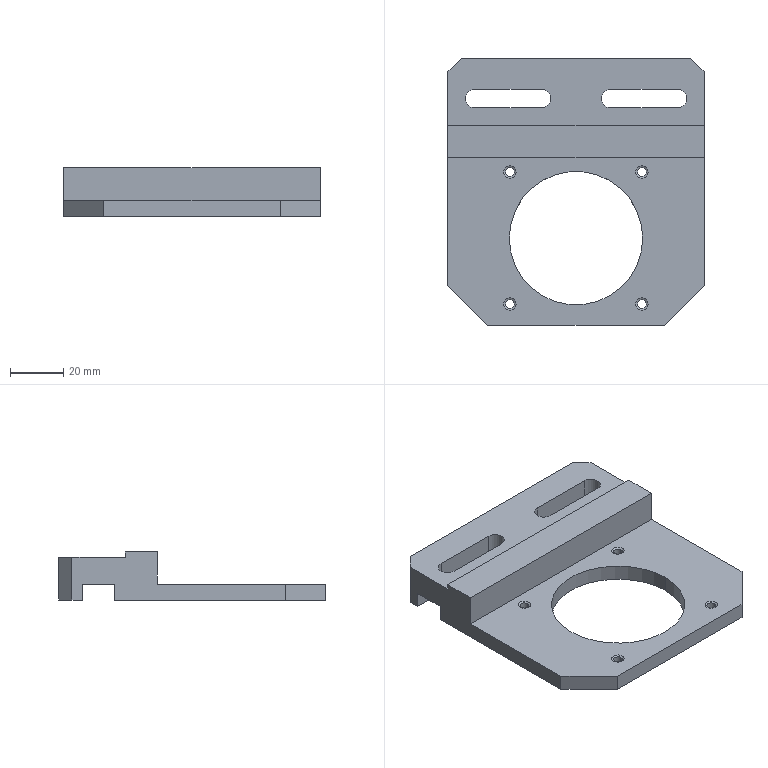Part | NX | 1 solid | 46 faces | box 96 x 100 x 18 mm | volume 70500 mm3 | plane 22 | cylinder 16 | cone 8 | commonest cylinder face diameters 3.3 x8 7 x6 50 x2
STEP:
#1=CARTESIAN_POINT('',(48.,41.,-8.));
#2=VERTEX_POINT('',#1);
#3=CARTESIAN_POINT('',(48.,45.,-8.));
#4=VERTEX_POINT('',#3);
#5=CARTESIAN_POINT('',(48.,0.,-8.));
#6=DIRECTION('',(0.,1.,0.));
#7=VECTOR('',#6,1000.);
#8=LINE('',#5,#7);
#9=EDGE_CURVE('',#2,#4,#8,.T.);
#10=ORIENTED_EDGE('',*,*,#9,.F.);
#11=CARTESIAN_POINT('',(-48.,41.,-8.));
#12=VERTEX_POINT('',#11);
#13=CARTESIAN_POINT('',(0.,41.,-8.));
#14=DIRECTION('',(-1.,0.,0.));
#15=VECTOR('',#14,1000.);
#16=LINE('',#13,#15);
#17=EDGE_CURVE('',#2,#12,#16,.T.);
#18=ORIENTED_EDGE('',*,*,#17,.T.);
#19=CARTESIAN_POINT('',(-48.,45.,-8.));
#20=VERTEX_POINT('',#19);
#21=CARTESIAN_POINT('',(-48.,0.,-8.));
#22=DIRECTION('',(0.,1.,0.));
#23=VECTOR('',#22,1000.);
#24=LINE('',#21,#23);
#25=EDGE_CURVE('',#12,#20,#24,.T.);
#26=ORIENTED_EDGE('',*,*,#25,.T.);
#27=CARTESIAN_POINT('',(-43.,50.,-8.));
#28=VERTEX_POINT('',#27);
#29=CARTESIAN_POINT('',(-93.,0.,-8.));
#30=DIRECTION('',(0.7071,0.7071,0.));
#31=VECTOR('',#30,1000.);
#32=LINE('',#29,#31);
#33=EDGE_CURVE('',#20,#28,#32,.T.);
#34=ORIENTED_EDGE('',*,*,#33,.T.);
#35=CARTESIAN_POINT('',(43.,50.,-8.));
#36=VERTEX_POINT('',#35);
#37=CARTESIAN_POINT('',(0.,50.,-8.));
#38=DIRECTION('',(-1.,0.,0.));
#39=VECTOR('',#38,1000.);
#40=LINE('',#37,#39);
#41=EDGE_CURVE('',#36,#28,#40,.T.);
#42=ORIENTED_EDGE('',*,*,#41,.F.);
#43=CARTESIAN_POINT('',(93.,0.,-8.));
#44=DIRECTION('',(0.7071,-0.7071,0.));
#45=VECTOR('',#44,1000.);
#46=LINE('',#43,#45);
#47=EDGE_CURVE('',#36,#4,#46,.T.);
#48=ORIENTED_EDGE('',*,*,#47,.T.);
#49=EDGE_LOOP('',(#10,#18,#26,#34,#42,#48));
#50=FACE_BOUND('',#49,.T.);
#51=CARTESIAN_POINT('',(0.,0.,-8.));
#52=DIRECTION('',(0.,0.,1.));
#53=DIRECTION('',(1.,0.,0.));
#54=AXIS2_PLACEMENT_3D('',#51,#52,#53);
#55=PLANE('',#54);
#56=ADVANCED_FACE('',(#50),#55,.F.);
#57=CARTESIAN_POINT('',(-48.,45.,8.));
#58=VERTEX_POINT('',#57);
#59=CARTESIAN_POINT('',(-48.,45.,0.));
#60=DIRECTION('',(0.,0.,1.));
#61=VECTOR('',#60,1000.);
#62=LINE('',#59,#61);
#63=EDGE_CURVE('',#20,#58,#62,.T.);
#64=ORIENTED_EDGE('',*,*,#63,.F.);
#65=ORIENTED_EDGE('',*,*,#25,.F.);
#66=CARTESIAN_POINT('',(-48.,41.,-2.));
#67=VERTEX_POINT('',#66);
#68=CARTESIAN_POINT('',(-48.,41.,0.));
#69=DIRECTION('',(0.,0.,-1.));
#70=VECTOR('',#69,1000.);
#71=LINE('',#68,#70);
#72=EDGE_CURVE('',#67,#12,#71,.T.);
#73=ORIENTED_EDGE('',*,*,#72,.F.);
#74=CARTESIAN_POINT('',(-48.,29.,-2.));
#75=VERTEX_POINT('',#74);
#76=CARTESIAN_POINT('',(-48.,0.,-2.));
#77=DIRECTION('',(0.,-1.,0.));
#78=VECTOR('',#77,1000.);
#79=LINE('',#76,#78);
#80=EDGE_CURVE('',#67,#75,#79,.T.);
#81=ORIENTED_EDGE('',*,*,#80,.T.);
#82=CARTESIAN_POINT('',(-48.,29.,-8.));
#83=VERTEX_POINT('',#82);
#84=CARTESIAN_POINT('',(-48.,29.,0.));
#85=DIRECTION('',(0.,0.,1.));
#86=VECTOR('',#85,1000.);
#87=LINE('',#84,#86);
#88=EDGE_CURVE('',#83,#75,#87,.T.);
#89=ORIENTED_EDGE('',*,*,#88,.F.);
#90=CARTESIAN_POINT('',(-48.,-35.,-8.));
#91=VERTEX_POINT('',#90);
#92=CARTESIAN_POINT('',(-48.,0.,-8.));
#93=DIRECTION('',(0.,1.,0.));
#94=VECTOR('',#93,1000.);
#95=LINE('',#92,#94);
#96=EDGE_CURVE('',#91,#83,#95,.T.);
#97=ORIENTED_EDGE('',*,*,#96,.F.);
#98=CARTESIAN_POINT('',(-48.,-35.,-2.));
#99=VERTEX_POINT('',#98);
#100=CARTESIAN_POINT('',(-48.,-35.,0.));
#101=DIRECTION('',(0.,0.,-1.));
#102=VECTOR('',#101,1000.);
#103=LINE('',#100,#102);
#104=EDGE_CURVE('',#99,#91,#103,.T.);
#105=ORIENTED_EDGE('',*,*,#104,.F.);
#106=CARTESIAN_POINT('',(-48.,13.,-2.));
#107=VERTEX_POINT('',#106);
#108=CARTESIAN_POINT('',(-48.,0.,-2.));
#109=DIRECTION('',(0.,1.,0.));
#110=VECTOR('',#109,1000.);
#111=LINE('',#108,#110);
#112=EDGE_CURVE('',#99,#107,#111,.T.);
#113=ORIENTED_EDGE('',*,*,#112,.T.);
#114=CARTESIAN_POINT('',(-48.,13.,10.));
#115=VERTEX_POINT('',#114);
#116=CARTESIAN_POINT('',(-48.,13.,0.));
#117=DIRECTION('',(0.,0.,1.));
#118=VECTOR('',#117,1000.);
#119=LINE('',#116,#118);
#120=EDGE_CURVE('',#107,#115,#119,.T.);
#121=ORIENTED_EDGE('',*,*,#120,.T.);
#122=CARTESIAN_POINT('',(-48.,25.,10.));
#123=VERTEX_POINT('',#122);
#124=CARTESIAN_POINT('',(-48.,0.,10.));
#125=DIRECTION('',(0.,-1.,0.));
#126=VECTOR('',#125,1000.);
#127=LINE('',#124,#126);
#128=EDGE_CURVE('',#123,#115,#127,.T.);
#129=ORIENTED_EDGE('',*,*,#128,.F.);
#130=CARTESIAN_POINT('',(-48.,25.,8.));
#131=VERTEX_POINT('',#130);
#132=CARTESIAN_POINT('',(-48.,25.,0.));
#133=DIRECTION('',(0.,0.,1.));
#134=VECTOR('',#133,1000.);
#135=LINE('',#132,#134);
#136=EDGE_CURVE('',#131,#123,#135,.T.);
#137=ORIENTED_EDGE('',*,*,#136,.F.);
#138=CARTESIAN_POINT('',(-48.,0.,8.));
#139=DIRECTION('',(0.,1.,0.));
#140=VECTOR('',#139,1000.);
#141=LINE('',#138,#140);
#142=EDGE_CURVE('',#131,#58,#141,.T.);
#143=ORIENTED_EDGE('',*,*,#142,.T.);
#144=EDGE_LOOP('',(#64,#65,#73,#81,#89,#97,#105,#113,#121,#129,#137,#143));
#145=FACE_BOUND('',#144,.T.);
#146=CARTESIAN_POINT('',(-48.,50.,-8.));
#147=DIRECTION('',(-1.,0.,0.));
#148=DIRECTION('',(0.,0.,1.));
#149=AXIS2_PLACEMENT_3D('',#146,#147,#148);
#150=PLANE('',#149);
#151=ADVANCED_FACE('',(#145),#150,.T.);
#152=CARTESIAN_POINT('',(43.,50.,8.));
#153=VERTEX_POINT('',#152);
#154=CARTESIAN_POINT('',(-43.,50.,8.));
#155=VERTEX_POINT('',#154);
#156=CARTESIAN_POINT('',(0.,50.,8.));
#157=DIRECTION('',(-1.,0.,0.));
#158=VECTOR('',#157,1000.);
#159=LINE('',#156,#158);
#160=EDGE_CURVE('',#153,#155,#159,.T.);
#161=ORIENTED_EDGE('',*,*,#160,.T.);
#162=CARTESIAN_POINT('',(-93.,0.,8.));
#163=DIRECTION('',(0.7071,0.7071,0.));
#164=VECTOR('',#163,1000.);
#165=LINE('',#162,#164);
#166=EDGE_CURVE('',#58,#155,#165,.T.);
#167=ORIENTED_EDGE('',*,*,#166,.F.);
#168=ORIENTED_EDGE('',*,*,#142,.F.);
#169=CARTESIAN_POINT('',(48.,25.,8.));
#170=VERTEX_POINT('',#169);
#171=CARTESIAN_POINT('',(0.,25.,8.));
#172=DIRECTION('',(1.,0.,0.));
#173=VECTOR('',#172,1000.);
#174=LINE('',#171,#173);
#175=EDGE_CURVE('',#131,#170,#174,.T.);
#176=ORIENTED_EDGE('',*,*,#175,.T.);
#177=CARTESIAN_POINT('',(48.,45.,8.));
#178=VERTEX_POINT('',#177);
#179=CARTESIAN_POINT('',(48.,0.,8.));
#180=DIRECTION('',(0.,1.,0.));
#181=VECTOR('',#180,1000.);
#182=LINE('',#179,#181);
#183=EDGE_CURVE('',#170,#178,#182,.T.);
#184=ORIENTED_EDGE('',*,*,#183,.T.);
#185=CARTESIAN_POINT('',(93.,0.,8.));
#186=DIRECTION('',(0.7071,-0.7071,0.));
#187=VECTOR('',#186,1000.);
#188=LINE('',#185,#187);
#189=EDGE_CURVE('',#153,#178,#188,.T.);
#190=ORIENTED_EDGE('',*,*,#189,.F.);
#191=EDGE_LOOP('',(#161,#167,#168,#176,#184,#190));
#192=FACE_BOUND('',#191,.T.);
#193=CARTESIAN_POINT('',(-13.,31.5,8.));
#194=VERTEX_POINT('',#193);
#195=CARTESIAN_POINT('',(-38.,31.5,8.));
#196=VERTEX_POINT('',#195);
#197=CARTESIAN_POINT('',(0.,31.5,8.));
#198=DIRECTION('',(-1.,0.,0.));
#199=VECTOR('',#198,1000.);
#200=LINE('',#197,#199);
#201=EDGE_CURVE('',#194,#196,#200,.T.);
#202=ORIENTED_EDGE('',*,*,#201,.T.);
#203=CARTESIAN_POINT('',(-41.5,35.,8.));
#204=VERTEX_POINT('',#203);
#205=CARTESIAN_POINT('',(-38.,35.,8.));
#206=DIRECTION('',(0.,0.,-1.));
#207=DIRECTION('',(-1.,0.,0.));
#208=AXIS2_PLACEMENT_3D('',#205,#206,#207);
#209=CIRCLE('',#208,3.5);
#210=EDGE_CURVE('',#196,#204,#209,.T.);
#211=ORIENTED_EDGE('',*,*,#210,.T.);
#212=CARTESIAN_POINT('',(-38.,38.5,8.));
#213=VERTEX_POINT('',#212);
#214=CARTESIAN_POINT('',(-38.,35.,8.));
#215=DIRECTION('',(0.,0.,-1.));
#216=DIRECTION('',(-1.,0.,0.));
#217=AXIS2_PLACEMENT_3D('',#214,#215,#216);
#218=CIRCLE('',#217,3.5);
#219=EDGE_CURVE('',#204,#213,#218,.T.);
#220=ORIENTED_EDGE('',*,*,#219,.T.);
#221=CARTESIAN_POINT('',(-13.,38.5,8.));
#222=VERTEX_POINT('',#221);
#223=CARTESIAN_POINT('',(0.,38.5,8.));
#224=DIRECTION('',(1.,0.,0.));
#225=VECTOR('',#224,1000.);
#226=LINE('',#223,#225);
#227=EDGE_CURVE('',#213,#222,#226,.T.);
#228=ORIENTED_EDGE('',*,*,#227,.T.);
#229=CARTESIAN_POINT('',(-13.,35.,8.));
#230=DIRECTION('',(0.,0.,-1.));
#231=DIRECTION('',(-1.,0.,0.));
#232=AXIS2_PLACEMENT_3D('',#229,#230,#231);
#233=CIRCLE('',#232,3.5);
#234=EDGE_CURVE('',#222,#194,#233,.T.);
#235=ORIENTED_EDGE('',*,*,#234,.T.);
#236=EDGE_LOOP('',(#202,#211,#220,#228,#235));
#237=FACE_BOUND('',#236,.T.);
#238=CARTESIAN_POINT('',(38.,31.5,8.));
#239=VERTEX_POINT('',#238);
#240=CARTESIAN_POINT('',(13.,31.5,8.));
#241=VERTEX_POINT('',#240);
#242=CARTESIAN_POINT('',(0.,31.5,8.));
#243=DIRECTION('',(-1.,0.,0.));
#244=VECTOR('',#243,1000.);
#245=LINE('',#242,#244);
#246=EDGE_CURVE('',#239,#241,#245,.T.);
#247=ORIENTED_EDGE('',*,*,#246,.T.);
#248=CARTESIAN_POINT('',(9.5,35.,8.));
#249=VERTEX_POINT('',#248);
#250=CARTESIAN_POINT('',(13.,35.,8.));
#251=DIRECTION('',(0.,0.,-1.));
#252=DIRECTION('',(-1.,0.,0.));
#253=AXIS2_PLACEMENT_3D('',#250,#251,#252);
#254=CIRCLE('',#253,3.5);
#255=EDGE_CURVE('',#241,#249,#254,.T.);
#256=ORIENTED_EDGE('',*,*,#255,.T.);
#257=CARTESIAN_POINT('',(13.,38.5,8.));
#258=VERTEX_POINT('',#257);
#259=CARTESIAN_POINT('',(13.,35.,8.));
#260=DIRECTION('',(0.,0.,-1.));
#261=DIRECTION('',(-1.,0.,0.));
#262=AXIS2_PLACEMENT_3D('',#259,#260,#261);
#263=CIRCLE('',#262,3.5);
#264=EDGE_CURVE('',#249,#258,#263,.T.);
#265=ORIENTED_EDGE('',*,*,#264,.T.);
#266=CARTESIAN_POINT('',(38.,38.5,8.));
#267=VERTEX_POINT('',#266);
#268=CARTESIAN_POINT('',(0.,38.5,8.));
#269=DIRECTION('',(1.,0.,0.));
#270=VECTOR('',#269,1000.);
#271=LINE('',#268,#270);
#272=EDGE_CURVE('',#258,#267,#271,.T.);
#273=ORIENTED_EDGE('',*,*,#272,.T.);
#274=CARTESIAN_POINT('',(38.,35.,8.));
#275=DIRECTION('',(0.,0.,-1.));
#276=DIRECTION('',(-1.,0.,0.));
#277=AXIS2_PLACEMENT_3D('',#274,#275,#276);
#278=CIRCLE('',#277,3.5);
#279=EDGE_CURVE('',#267,#239,#278,.T.);
#280=ORIENTED_EDGE('',*,*,#279,.T.);
#281=EDGE_LOOP('',(#247,#256,#265,#273,#280));
#282=FACE_BOUND('',#281,.T.);
#283=CARTESIAN_POINT('',(0.,0.,8.));
#284=DIRECTION('',(0.,0.,1.));
#285=DIRECTION('',(1.,0.,0.));
#286=AXIS2_PLACEMENT_3D('',#283,#284,#285);
#287=PLANE('',#286);
#288=ADVANCED_FACE('',(#192,#237,#282),#287,.T.);
#289=ORIENTED_EDGE('',*,*,#175,.F.);
#290=ORIENTED_EDGE('',*,*,#136,.T.);
#291=CARTESIAN_POINT('',(48.,25.,10.));
#292=VERTEX_POINT('',#291);
#293=CARTESIAN_POINT('',(48.,25.,10.));
#294=DIRECTION('',(-1.,0.,0.));
#295=VECTOR('',#294,1000.);
#296=LINE('',#293,#295);
#297=EDGE_CURVE('',#292,#123,#296,.T.);
#298=ORIENTED_EDGE('',*,*,#297,.F.);
#299=CARTESIAN_POINT('',(48.,25.,0.));
#300=DIRECTION('',(0.,0.,-1.));
#301=VECTOR('',#300,1000.);
#302=LINE('',#299,#301);
#303=EDGE_CURVE('',#292,#170,#302,.T.);
#304=ORIENTED_EDGE('',*,*,#303,.T.);
#305=EDGE_LOOP('',(#289,#290,#298,#304));
#306=FACE_BOUND('',#305,.T.);
#307=CARTESIAN_POINT('',(-48.,25.,8.));
#308=DIRECTION('',(0.,1.,0.));
#309=DIRECTION('',(1.,0.,0.));
#310=AXIS2_PLACEMENT_3D('',#307,#308,#309);
#311=PLANE('',#310);
#312=ADVANCED_FACE('',(#306),#311,.T.);
#313=CARTESIAN_POINT('',(48.,45.,0.));
#314=DIRECTION('',(0.,0.,-1.));
#315=VECTOR('',#314,1000.);
#316=LINE('',#313,#315);
#317=EDGE_CURVE('',#178,#4,#316,.T.);
#318=ORIENTED_EDGE('',*,*,#317,.F.);
#319=ORIENTED_EDGE('',*,*,#183,.F.);
#320=ORIENTED_EDGE('',*,*,#303,.F.);
#321=CARTESIAN_POINT('',(48.,13.,10.));
#322=VERTEX_POINT('',#321);
#323=CARTESIAN_POINT('',(48.,0.,10.));
#324=DIRECTION('',(0.,1.,0.));
#325=VECTOR('',#324,1000.);
#326=LINE('',#323,#325);
#327=EDGE_CURVE('',#322,#292,#326,.T.);
#328=ORIENTED_EDGE('',*,*,#327,.F.);
#329=CARTESIAN_POINT('',(48.,13.,-2.));
#330=VERTEX_POINT('',#329);
#331=CARTESIAN_POINT('',(48.,13.,0.));
#332=DIRECTION('',(0.,0.,-1.));
#333=VECTOR('',#332,1000.);
#334=LINE('',#331,#333);
#335=EDGE_CURVE('',#322,#330,#334,.T.);
#336=ORIENTED_EDGE('',*,*,#335,.T.);
#337=CARTESIAN_POINT('',(48.,-35.,-2.));
#338=VERTEX_POINT('',#337);
#339=CARTESIAN_POINT('',(48.,0.,-2.));
#340=DIRECTION('',(0.,-1.,0.));
#341=VECTOR('',#340,1000.);
#342=LINE('',#339,#341);
#343=EDGE_CURVE('',#330,#338,#342,.T.);
#344=ORIENTED_EDGE('',*,*,#343,.T.);
#345=CARTESIAN_POINT('',(48.,-35.,-8.));
#346=VERTEX_POINT('',#345);
#347=CARTESIAN_POINT('',(48.,-35.,0.));
#348=DIRECTION('',(0.,0.,1.));
#349=VECTOR('',#348,1000.);
#350=LINE('',#347,#349);
#351=EDGE_CURVE('',#346,#338,#350,.T.);
#352=ORIENTED_EDGE('',*,*,#351,.F.);
#353=CARTESIAN_POINT('',(48.,29.,-8.));
#354=VERTEX_POINT('',#353);
#355=CARTESIAN_POINT('',(48.,0.,-8.));
#356=DIRECTION('',(0.,1.,0.));
#357=VECTOR('',#356,1000.);
#358=LINE('',#355,#357);
#359=EDGE_CURVE('',#346,#354,#358,.T.);
#360=ORIENTED_EDGE('',*,*,#359,.T.);
#361=CARTESIAN_POINT('',(48.,29.,-2.));
#362=VERTEX_POINT('',#361);
#363=CARTESIAN_POINT('',(48.,29.,0.));
#364=DIRECTION('',(0.,0.,-1.));
#365=VECTOR('',#364,1000.);
#366=LINE('',#363,#365);
#367=EDGE_CURVE('',#362,#354,#366,.T.);
#368=ORIENTED_EDGE('',*,*,#367,.F.);
#369=CARTESIAN_POINT('',(48.,41.,-2.));
#370=VERTEX_POINT('',#369);
#371=CARTESIAN_POINT('',(48.,0.,-2.));
#372=DIRECTION('',(0.,1.,0.));
#373=VECTOR('',#372,1000.);
#374=LINE('',#371,#373);
#375=EDGE_CURVE('',#362,#370,#374,.T.);
#376=ORIENTED_EDGE('',*,*,#375,.T.);
#377=CARTESIAN_POINT('',(48.,41.,0.));
#378=DIRECTION('',(0.,0.,1.));
#379=VECTOR('',#378,1000.);
#380=LINE('',#377,#379);
#381=EDGE_CURVE('',#2,#370,#380,.T.);
#382=ORIENTED_EDGE('',*,*,#381,.F.);
#383=ORIENTED_EDGE('',*,*,#9,.T.);
#384=EDGE_LOOP('',(#318,#319,#320,#328,#336,#344,#352,#360,#368,#376,#382,#383));
#385=FACE_BOUND('',#384,.T.);
#386=CARTESIAN_POINT('',(48.,-50.,-8.));
#387=DIRECTION('',(1.,0.,0.));
#388=DIRECTION('',(0.,1.,0.));
#389=AXIS2_PLACEMENT_3D('',#386,#387,#388);
#390=PLANE('',#389);
#391=ADVANCED_FACE('',(#385),#390,.T.);
#392=ORIENTED_EDGE('',*,*,#120,.F.);
#393=CARTESIAN_POINT('',(0.,13.,-2.));
#394=DIRECTION('',(-1.,0.,0.));
#395=VECTOR('',#394,1000.);
#396=LINE('',#393,#395);
#397=EDGE_CURVE('',#330,#107,#396,.T.);
#398=ORIENTED_EDGE('',*,*,#397,.F.);
#399=ORIENTED_EDGE('',*,*,#335,.F.);
#400=CARTESIAN_POINT('',(48.,13.,10.));
#401=DIRECTION('',(-1.,0.,0.));
#402=VECTOR('',#401,1000.);
#403=LINE('',#400,#402);
#404=EDGE_CURVE('',#322,#115,#403,.T.);
#405=ORIENTED_EDGE('',*,*,#404,.T.);
#406=EDGE_LOOP('',(#392,#398,#399,#405));
#407=FACE_BOUND('',#406,.T.);
#408=CARTESIAN_POINT('',(48.,13.,-2.));
#409=DIRECTION('',(0.,1.,0.));
#410=DIRECTION('',(1.,0.,0.));
#411=AXIS2_PLACEMENT_3D('',#408,#409,#410);
#412=PLANE('',#411);
#413=ADVANCED_FACE('',(#407),#412,.F.);
#414=ORIENTED_EDGE('',*,*,#128,.T.);
#415=ORIENTED_EDGE('',*,*,#404,.F.);
#416=ORIENTED_EDGE('',*,*,#327,.T.);
#417=ORIENTED_EDGE('',*,*,#297,.T.);
#418=EDGE_LOOP('',(#414,#415,#416,#417));
#419=FACE_BOUND('',#418,.T.);
#420=CARTESIAN_POINT('',(-48.,25.,10.));
#421=DIRECTION('',(0.,0.,1.));
#422=DIRECTION('',(1.,0.,0.));
#423=AXIS2_PLACEMENT_3D('',#420,#421,#422);
#424=PLANE('',#423);
#425=ADVANCED_FACE('',(#419),#424,.T.);
#426=ORIENTED_EDGE('',*,*,#112,.F.);
#427=CARTESIAN_POINT('',(-33.,-50.,-2.));
#428=VERTEX_POINT('',#427);
#429=CARTESIAN_POINT('',(-83.,0.,-2.));
#430=DIRECTION('',(0.7071,-0.7071,0.));
#431=VECTOR('',#430,1000.);
#432=LINE('',#429,#431);
#433=EDGE_CURVE('',#99,#428,#432,.T.);
#434=ORIENTED_EDGE('',*,*,#433,.T.);
#435=CARTESIAN_POINT('',(33.,-50.,-2.));
#436=VERTEX_POINT('',#435);
#437=CARTESIAN_POINT('',(0.,-50.,-2.));
#438=DIRECTION('',(1.,0.,0.));
#439=VECTOR('',#438,1000.);
#440=LINE('',#437,#439);
#441=EDGE_CURVE('',#428,#436,#440,.T.);
#442=ORIENTED_EDGE('',*,*,#441,.T.);
#443=CARTESIAN_POINT('',(83.,0.,-2.));
#444=DIRECTION('',(0.7071,0.7071,0.));
#445=VECTOR('',#444,1000.);
#446=LINE('',#443,#445);
#447=EDGE_CURVE('',#436,#338,#446,.T.);
#448=ORIENTED_EDGE('',*,*,#447,.T.);
#449=ORIENTED_EDGE('',*,*,#343,.F.);
#450=ORIENTED_EDGE('',*,*,#397,.T.);
#451=EDGE_LOOP('',(#426,#434,#442,#448,#449,#450));
#452=FACE_BOUND('',#451,.T.);
#453=CARTESIAN_POINT('',(25.,-17.3,-2.));
#454=VERTEX_POINT('',#453);
#455=CARTESIAN_POINT('',(-25.,-17.3,-2.));
#456=VERTEX_POINT('',#455);
#457=CARTESIAN_POINT('',(0.,-17.3,-2.));
#458=DIRECTION('',(0.,0.,-1.));
#459=DIRECTION('',(-1.,0.,0.));
#460=AXIS2_PLACEMENT_3D('',#457,#458,#459);
#461=CIRCLE('',#460,25.);
#462=EDGE_CURVE('',#454,#456,#461,.T.);
#463=ORIENTED_EDGE('',*,*,#462,.T.);
#464=CARTESIAN_POINT('',(0.,-17.3,-2.));
#465=DIRECTION('',(0.,0.,-1.));
#466=DIRECTION('',(-1.,0.,0.));
#467=AXIS2_PLACEMENT_3D('',#464,#465,#466);
#468=CIRCLE('',#467,25.);
#469=EDGE_CURVE('',#456,#454,#468,.T.);
#470=ORIENTED_EDGE('',*,*,#469,.T.);
#471=EDGE_LOOP('',(#463,#470));
#472=FACE_BOUND('',#471,.T.);
#473=CARTESIAN_POINT('',(-27.112,7.499,-2.));
#474=VERTEX_POINT('',#473);
#475=CARTESIAN_POINT('',(-22.482,7.499,-2.));
#476=VERTEX_POINT('',#475);
#477=CARTESIAN_POINT('',(-24.797,7.499,-2.));
#478=DIRECTION('',(0.,0.,1.));
#479=DIRECTION('',(1.,0.,0.));
#480=AXIS2_PLACEMENT_3D('',#477,#478,#479);
#481=CIRCLE('',#480,2.315);
#482=EDGE_CURVE('',#474,#476,#481,.T.);
#483=ORIENTED_EDGE('',*,*,#482,.F.);
#484=CARTESIAN_POINT('',(-24.797,7.499,-2.));
#485=DIRECTION('',(0.,0.,1.));
#486=DIRECTION('',(1.,0.,0.));
#487=AXIS2_PLACEMENT_3D('',#484,#485,#486);
#488=CIRCLE('',#487,2.315);
#489=EDGE_CURVE('',#476,#474,#488,.T.);
#490=ORIENTED_EDGE('',*,*,#489,.F.);
#491=EDGE_LOOP('',(#483,#490));
#492=FACE_BOUND('',#491,.T.);
#493=CARTESIAN_POINT('',(27.015,-41.999,-2.));
#494=VERTEX_POINT('',#493);
#495=CARTESIAN_POINT('',(22.385,-41.999,-2.));
#496=VERTEX_POINT('',#495);
#497=CARTESIAN_POINT('',(24.7,-41.999,-2.));
#498=DIRECTION('',(0.,0.,1.));
#499=DIRECTION('',(1.,0.,0.));
#500=AXIS2_PLACEMENT_3D('',#497,#498,#499);
#501=CIRCLE('',#500,2.315);
#502=EDGE_CURVE('',#494,#496,#501,.T.);
#503=ORIENTED_EDGE('',*,*,#502,.F.);
#504=CARTESIAN_POINT('',(24.7,-41.999,-2.));
#505=DIRECTION('',(0.,0.,1.));
#506=DIRECTION('',(1.,0.,0.));
#507=AXIS2_PLACEMENT_3D('',#504,#505,#506);
#508=CIRCLE('',#507,2.315);
#509=EDGE_CURVE('',#496,#494,#508,.T.);
#510=ORIENTED_EDGE('',*,*,#509,.F.);
#511=EDGE_LOOP('',(#503,#510));
#512=FACE_BOUND('',#511,.T.);
#513=CARTESIAN_POINT('',(-22.482,-41.999,-2.));
#514=VERTEX_POINT('',#513);
#515=CARTESIAN_POINT('',(-27.112,-41.999,-2.));
#516=VERTEX_POINT('',#515);
#517=CARTESIAN_POINT('',(-24.797,-41.999,-2.));
#518=DIRECTION('',(0.,0.,1.));
#519=DIRECTION('',(1.,0.,0.));
#520=AXIS2_PLACEMENT_3D('',#517,#518,#519);
#521=CIRCLE('',#520,2.315);
#522=EDGE_CURVE('',#514,#516,#521,.T.);
#523=ORIENTED_EDGE('',*,*,#522,.F.);
#524=CARTESIAN_POINT('',(-24.797,-41.999,-2.));
#525=DIRECTION('',(0.,0.,1.));
#526=DIRECTION('',(1.,0.,0.));
#527=AXIS2_PLACEMENT_3D('',#524,#525,#526);
#528=CIRCLE('',#527,2.315);
#529=EDGE_CURVE('',#516,#514,#528,.T.);
#530=ORIENTED_EDGE('',*,*,#529,.F.);
#531=EDGE_LOOP('',(#523,#530));
#532=FACE_BOUND('',#531,.T.);
#533=CARTESIAN_POINT('',(27.015,7.499,-2.));
#534=VERTEX_POINT('',#533);
#535=CARTESIAN_POINT('',(22.385,7.499,-2.));
#536=VERTEX_POINT('',#535);
#537=CARTESIAN_POINT('',(24.7,7.499,-2.));
#538=DIRECTION('',(0.,0.,1.));
#539=DIRECTION('',(1.,0.,0.));
#540=AXIS2_PLACEMENT_3D('',#537,#538,#539);
#541=CIRCLE('',#540,2.315);
#542=EDGE_CURVE('',#534,#536,#541,.T.);
#543=ORIENTED_EDGE('',*,*,#542,.F.);
#544=CARTESIAN_POINT('',(24.7,7.499,-2.));
#545=DIRECTION('',(0.,0.,1.));
#546=DIRECTION('',(1.,0.,0.));
#547=AXIS2_PLACEMENT_3D('',#544,#545,#546);
#548=CIRCLE('',#547,2.315);
#549=EDGE_CURVE('',#536,#534,#548,.T.);
#550=ORIENTED_EDGE('',*,*,#549,.F.);
#551=EDGE_LOOP('',(#543,#550));
#552=FACE_BOUND('',#551,.T.);
#553=CARTESIAN_POINT('',(48.,-50.,-2.));
#554=DIRECTION('',(0.,0.,-1.));
#555=DIRECTION('',(0.,-1.,0.));
#556=AXIS2_PLACEMENT_3D('',#553,#554,#555);
#557=PLANE('',#556);
#558=ADVANCED_FACE('',(#452,#472,#492,#512,#532,#552),#557,.F.);
#559=ORIENTED_EDGE('',*,*,#447,.F.);
#560=CARTESIAN_POINT('',(33.,-50.,-8.));
#561=VERTEX_POINT('',#560);
#562=CARTESIAN_POINT('',(33.,-50.,-2.));
#563=DIRECTION('',(0.,0.,-1.));
#564=VECTOR('',#563,1000.);
#565=LINE('',#562,#564);
#566=EDGE_CURVE('',#436,#561,#565,.T.);
#567=ORIENTED_EDGE('',*,*,#566,.T.);
#568=CARTESIAN_POINT('',(83.,0.,-8.));
#569=DIRECTION('',(-0.7071,-0.7071,0.));
#570=VECTOR('',#569,1000.);
#571=LINE('',#568,#570);
#572=EDGE_CURVE('',#346,#561,#571,.T.);
#573=ORIENTED_EDGE('',*,*,#572,.F.);
#574=ORIENTED_EDGE('',*,*,#351,.T.);
#575=EDGE_LOOP('',(#559,#567,#573,#574));
#576=FACE_BOUND('',#575,.T.);
#577=CARTESIAN_POINT('',(48.,-35.,-8.));
#578=DIRECTION('',(0.7071,-0.7071,0.));
#579=DIRECTION('',(0.,0.,-1.));
#580=AXIS2_PLACEMENT_3D('',#577,#578,#579);
#581=PLANE('',#580);
#582=ADVANCED_FACE('',(#576),#581,.T.);
#583=ORIENTED_EDGE('',*,*,#441,.F.);
#584=CARTESIAN_POINT('',(-33.,-50.,-8.));
#585=VERTEX_POINT('',#584);
#586=CARTESIAN_POINT('',(-33.,-50.,-2.));
#587=DIRECTION('',(0.,0.,-1.));
#588=VECTOR('',#587,1000.);
#589=LINE('',#586,#588);
#590=EDGE_CURVE('',#428,#585,#589,.T.);
#591=ORIENTED_EDGE('',*,*,#590,.T.);
#592=CARTESIAN_POINT('',(0.,-50.,-8.));
#593=DIRECTION('',(-1.,0.,0.));
#594=VECTOR('',#593,1000.);
#595=LINE('',#592,#594);
#596=EDGE_CURVE('',#561,#585,#595,.T.);
#597=ORIENTED_EDGE('',*,*,#596,.F.);
#598=ORIENTED_EDGE('',*,*,#566,.F.);
#599=EDGE_LOOP('',(#583,#591,#597,#598));
#600=FACE_BOUND('',#599,.T.);
#601=CARTESIAN_POINT('',(-48.,-50.,-8.));
#602=DIRECTION('',(0.,-1.,0.));
#603=DIRECTION('',(0.,0.,-1.));
#604=AXIS2_PLACEMENT_3D('',#601,#602,#603);
#605=PLANE('',#604);
#606=ADVANCED_FACE('',(#600),#605,.T.);
#607=ORIENTED_EDGE('',*,*,#433,.F.);
#608=ORIENTED_EDGE('',*,*,#104,.T.);
#609=CARTESIAN_POINT('',(-83.,0.,-8.));
#610=DIRECTION('',(-0.7071,0.7071,0.));
#611=VECTOR('',#610,1000.);
#612=LINE('',#609,#611);
#613=EDGE_CURVE('',#585,#91,#612,.T.);
#614=ORIENTED_EDGE('',*,*,#613,.F.);
#615=ORIENTED_EDGE('',*,*,#590,.F.);
#616=EDGE_LOOP('',(#607,#608,#614,#615));
#617=FACE_BOUND('',#616,.T.);
#618=CARTESIAN_POINT('',(-33.,-50.,-8.));
#619=DIRECTION('',(-0.7071,-0.7071,0.));
#620=DIRECTION('',(-0.7071,0.7071,0.));
#621=AXIS2_PLACEMENT_3D('',#618,#619,#620);
#622=PLANE('',#621);
#623=ADVANCED_FACE('',(#617),#622,.T.);
#624=ORIENTED_EDGE('',*,*,#462,.F.);
#625=CARTESIAN_POINT('',(25.,-17.3,-8.));
#626=VERTEX_POINT('',#625);
#627=CARTESIAN_POINT('',(25.,-17.3,8.));
#628=DIRECTION('',(0.,0.,-1.));
#629=VECTOR('',#628,1000.);
#630=LINE('',#627,#629);
#631=EDGE_CURVE('',#454,#626,#630,.T.);
#632=ORIENTED_EDGE('',*,*,#631,.T.);
#633=CARTESIAN_POINT('',(-25.,-17.3,-8.));
#634=VERTEX_POINT('',#633);
#635=CARTESIAN_POINT('',(0.,-17.3,-8.));
#636=DIRECTION('',(0.,0.,-1.));
#637=DIRECTION('',(-1.,0.,0.));
#638=AXIS2_PLACEMENT_3D('',#635,#636,#637);
#639=CIRCLE('',#638,25.);
#640=EDGE_CURVE('',#626,#634,#639,.T.);
#641=ORIENTED_EDGE('',*,*,#640,.T.);
#642=CARTESIAN_POINT('',(-25.,-17.3,8.));
#643=DIRECTION('',(0.,0.,-1.));
#644=VECTOR('',#643,1000.);
#645=LINE('',#642,#644);
#646=EDGE_CURVE('',#456,#634,#645,.T.);
#647=ORIENTED_EDGE('',*,*,#646,.F.);
#648=EDGE_LOOP('',(#624,#632,#641,#647));
#649=FACE_BOUND('',#648,.T.);
#650=CARTESIAN_POINT('',(0.,-17.3,8.));
#651=DIRECTION('',(0.,0.,-1.));
#652=DIRECTION('',(-1.,0.,0.));
#653=AXIS2_PLACEMENT_3D('',#650,#651,#652);
#654=CYLINDRICAL_SURFACE('',#653,25.);
#655=ADVANCED_FACE('',(#649),#654,.F.);
#656=ORIENTED_EDGE('',*,*,#502,.T.);
#657=CARTESIAN_POINT('',(23.05,-41.999,-2.384));
#658=VERTEX_POINT('',#657);
#659=CARTESIAN_POINT('',(23.05,-41.999,-2.384));
#660=DIRECTION('',(-0.866,0.,0.5));
#661=VECTOR('',#660,1000.);
#662=LINE('',#659,#661);
#663=EDGE_CURVE('',#658,#496,#662,.T.);
#664=ORIENTED_EDGE('',*,*,#663,.F.);
#665=CARTESIAN_POINT('',(26.35,-41.999,-2.384));
#666=VERTEX_POINT('',#665);
#667=CARTESIAN_POINT('',(24.7,-41.999,-2.384));
#668=DIRECTION('',(0.,0.,1.));
#669=DIRECTION('',(1.,0.,0.));
#670=AXIS2_PLACEMENT_3D('',#667,#668,#669);
#671=CIRCLE('',#670,1.65);
#672=EDGE_CURVE('',#666,#658,#671,.T.);
#673=ORIENTED_EDGE('',*,*,#672,.F.);
#674=CARTESIAN_POINT('',(26.35,-41.999,-2.384));
#675=DIRECTION('',(0.866,0.,0.5));
#676=VECTOR('',#675,1000.);
#677=LINE('',#674,#676);
#678=EDGE_CURVE('',#666,#494,#677,.T.);
#679=ORIENTED_EDGE('',*,*,#678,.T.);
#680=EDGE_LOOP('',(#656,#664,#673,#679));
#681=FACE_BOUND('',#680,.T.);
#682=CARTESIAN_POINT('',(24.7,-41.999,-2.384));
#683=DIRECTION('',(0.,0.,1.));
#684=DIRECTION('',(1.,0.,0.));
#685=AXIS2_PLACEMENT_3D('',#682,#683,#684);
#686=CONICAL_SURFACE('',#685,1.65,1.047);
#687=ADVANCED_FACE('',(#681),#686,.F.);
#688=ORIENTED_EDGE('',*,*,#542,.T.);
#689=CARTESIAN_POINT('',(23.05,7.499,-2.384));
#690=VERTEX_POINT('',#689);
#691=CARTESIAN_POINT('',(23.05,7.499,-2.384));
#692=DIRECTION('',(-0.866,0.,0.5));
#693=VECTOR('',#692,1000.);
#694=LINE('',#691,#693);
#695=EDGE_CURVE('',#536,#690,#694,.F.);
#696=ORIENTED_EDGE('',*,*,#695,.T.);
#697=CARTESIAN_POINT('',(26.35,7.499,-2.384));
#698=VERTEX_POINT('',#697);
#699=CARTESIAN_POINT('',(24.7,7.499,-2.384));
#700=DIRECTION('',(0.,0.,1.));
#701=DIRECTION('',(1.,0.,0.));
#702=AXIS2_PLACEMENT_3D('',#699,#700,#701);
#703=CIRCLE('',#702,1.65);
#704=EDGE_CURVE('',#698,#690,#703,.T.);
#705=ORIENTED_EDGE('',*,*,#704,.F.);
#706=CARTESIAN_POINT('',(26.35,7.499,-2.384));
#707=DIRECTION('',(0.866,0.,0.5));
#708=VECTOR('',#707,1000.);
#709=LINE('',#706,#708);
#710=EDGE_CURVE('',#534,#698,#709,.F.);
#711=ORIENTED_EDGE('',*,*,#710,.F.);
#712=EDGE_LOOP('',(#688,#696,#705,#711));
#713=FACE_BOUND('',#712,.T.);
#714=CARTESIAN_POINT('',(24.7,7.499,-2.384));
#715=DIRECTION('',(0.,0.,1.));
#716=DIRECTION('',(1.,0.,0.));
#717=AXIS2_PLACEMENT_3D('',#714,#715,#716);
#718=CONICAL_SURFACE('',#717,1.65,1.047);
#719=ADVANCED_FACE('',(#713),#718,.F.);
#720=CARTESIAN_POINT('',(23.05,-41.999,-8.));
#721=VERTEX_POINT('',#720);
#722=CARTESIAN_POINT('',(26.35,-41.999,-8.));
#723=VERTEX_POINT('',#722);
#724=CARTESIAN_POINT('',(24.7,-41.999,-8.));
#725=DIRECTION('',(0.,0.,1.));
#726=DIRECTION('',(1.,0.,0.));
#727=AXIS2_PLACEMENT_3D('',#724,#725,#726);
#728=CIRCLE('',#727,1.65);
#729=EDGE_CURVE('',#721,#723,#728,.T.);
#730=ORIENTED_EDGE('',*,*,#729,.F.);
#731=CARTESIAN_POINT('',(23.05,-41.999,-2.));
#732=DIRECTION('',(0.,0.,1.));
#733=VECTOR('',#732,1000.);
#734=LINE('',#731,#733);
#735=EDGE_CURVE('',#658,#721,#734,.F.);
#736=ORIENTED_EDGE('',*,*,#735,.F.);
#737=CARTESIAN_POINT('',(24.7,-41.999,-2.384));
#738=DIRECTION('',(0.,0.,1.));
#739=DIRECTION('',(1.,0.,0.));
#740=AXIS2_PLACEMENT_3D('',#737,#738,#739);
#741=CIRCLE('',#740,1.65);
#742=EDGE_CURVE('',#658,#666,#741,.T.);
#743=ORIENTED_EDGE('',*,*,#742,.T.);
#744=CARTESIAN_POINT('',(26.35,-41.999,-2.));
#745=DIRECTION('',(0.,0.,1.));
#746=VECTOR('',#745,1000.);
#747=LINE('',#744,#746);
#748=EDGE_CURVE('',#666,#723,#747,.F.);
#749=ORIENTED_EDGE('',*,*,#748,.T.);
#750=EDGE_LOOP('',(#730,#736,#743,#749));
#751=FACE_BOUND('',#750,.T.);
#752=CARTESIAN_POINT('',(24.7,-41.999,-2.));
#753=DIRECTION('',(0.,0.,1.));
#754=DIRECTION('',(1.,0.,0.));
#755=AXIS2_PLACEMENT_3D('',#752,#753,#754);
#756=CYLINDRICAL_SURFACE('',#755,1.65);
#757=ADVANCED_FACE('',(#751),#756,.F.);
#758=CARTESIAN_POINT('',(26.35,7.499,-8.));
#759=VERTEX_POINT('',#758);
#760=CARTESIAN_POINT('',(23.05,7.499,-8.));
#761=VERTEX_POINT('',#760);
#762=CARTESIAN_POINT('',(24.7,7.499,-8.));
#763=DIRECTION('',(0.,0.,1.));
#764=DIRECTION('',(1.,0.,0.));
#765=AXIS2_PLACEMENT_3D('',#762,#763,#764);
#766=CIRCLE('',#765,1.65);
#767=EDGE_CURVE('',#759,#761,#766,.T.);
#768=ORIENTED_EDGE('',*,*,#767,.F.);
#769=CARTESIAN_POINT('',(26.35,7.499,-2.));
#770=DIRECTION('',(0.,0.,1.));
#771=VECTOR('',#770,1000.);
#772=LINE('',#769,#771);
#773=EDGE_CURVE('',#759,#698,#772,.T.);
#774=ORIENTED_EDGE('',*,*,#773,.T.);
#775=ORIENTED_EDGE('',*,*,#704,.T.);
#776=CARTESIAN_POINT('',(23.05,7.499,-2.));
#777=DIRECTION('',(0.,0.,1.));
#778=VECTOR('',#777,1000.);
#779=LINE('',#776,#778);
#780=EDGE_CURVE('',#761,#690,#779,.T.);
#781=ORIENTED_EDGE('',*,*,#780,.F.);
#782=EDGE_LOOP('',(#768,#774,#775,#781));
#783=FACE_BOUND('',#782,.T.);
#784=CARTESIAN_POINT('',(24.7,7.499,-2.));
#785=DIRECTION('',(0.,0.,1.));
#786=DIRECTION('',(1.,0.,0.));
#787=AXIS2_PLACEMENT_3D('',#784,#785,#786);
#788=CYLINDRICAL_SURFACE('',#787,1.65);
#789=ADVANCED_FACE('',(#783),#788,.F.);
#790=ORIENTED_EDGE('',*,*,#482,.T.);
#791=CARTESIAN_POINT('',(-23.147,7.499,-2.384));
#792=VERTEX_POINT('',#791);
#793=CARTESIAN_POINT('',(-23.147,7.499,-2.384));
#794=DIRECTION('',(0.866,0.,0.5));
#795=VECTOR('',#794,1000.);
#796=LINE('',#793,#795);
#797=EDGE_CURVE('',#792,#476,#796,.T.);
#798=ORIENTED_EDGE('',*,*,#797,.F.);
#799=CARTESIAN_POINT('',(-26.447,7.499,-2.384));
#800=VERTEX_POINT('',#799);
#801=CARTESIAN_POINT('',(-24.797,7.499,-2.384));
#802=DIRECTION('',(0.,0.,1.));
#803=DIRECTION('',(1.,0.,0.));
#804=AXIS2_PLACEMENT_3D('',#801,#802,#803);
#805=CIRCLE('',#804,1.65);
#806=EDGE_CURVE('',#800,#792,#805,.T.);
#807=ORIENTED_EDGE('',*,*,#806,.F.);
#808=CARTESIAN_POINT('',(-26.447,7.499,-2.384));
#809=DIRECTION('',(-0.866,0.,0.5));
#810=VECTOR('',#809,1000.);
#811=LINE('',#808,#810);
#812=EDGE_CURVE('',#800,#474,#811,.T.);
#813=ORIENTED_EDGE('',*,*,#812,.T.);
#814=EDGE_LOOP('',(#790,#798,#807,#813));
#815=FACE_BOUND('',#814,.T.);
#816=CARTESIAN_POINT('',(-24.797,7.499,-2.384));
#817=DIRECTION('',(0.,0.,1.));
#818=DIRECTION('',(1.,0.,0.));
#819=AXIS2_PLACEMENT_3D('',#816,#817,#818);
#820=CONICAL_SURFACE('',#819,1.65,1.047);
#821=ADVANCED_FACE('',(#815),#820,.F.);
#822=ORIENTED_EDGE('',*,*,#246,.F.);
#823=CARTESIAN_POINT('',(38.,31.5,-2.));
#824=VERTEX_POINT('',#823);
#825=CARTESIAN_POINT('',(38.,31.5,11.8));
#826=DIRECTION('',(0.,0.,-1.));
#827=VECTOR('',#826,1000.);
#828=LINE('',#825,#827);
#829=EDGE_CURVE('',#239,#824,#828,.T.);
#830=ORIENTED_EDGE('',*,*,#829,.T.);
#831=CARTESIAN_POINT('',(13.,31.5,-2.));
#832=VERTEX_POINT('',#831);
#833=CARTESIAN_POINT('',(0.,31.5,-2.));
#834=DIRECTION('',(1.,0.,0.));
#835=VECTOR('',#834,1000.);
#836=LINE('',#833,#835);
#837=EDGE_CURVE('',#832,#824,#836,.T.);
#838=ORIENTED_EDGE('',*,*,#837,.F.);
#839=CARTESIAN_POINT('',(13.,31.5,11.8));
#840=DIRECTION('',(0.,0.,-1.));
#841=VECTOR('',#840,1000.);
#842=LINE('',#839,#841);
#843=EDGE_CURVE('',#241,#832,#842,.T.);
#844=ORIENTED_EDGE('',*,*,#843,.F.);
#845=EDGE_LOOP('',(#822,#830,#838,#844));
#846=FACE_BOUND('',#845,.T.);
#847=CARTESIAN_POINT('',(13.,31.5,11.8));
#848=DIRECTION('',(0.,-1.,0.));
#849=DIRECTION('',(0.,0.,-1.));
#850=AXIS2_PLACEMENT_3D('',#847,#848,#849);
#851=PLANE('',#850);
#852=ADVANCED_FACE('',(#846),#851,.F.);
#853=CARTESIAN_POINT('',(-26.447,-41.999,-2.384));
#854=VERTEX_POINT('',#853);
#855=CARTESIAN_POINT('',(-23.147,-41.999,-2.384));
#856=VERTEX_POINT('',#855);
#857=CARTESIAN_POINT('',(-24.797,-41.999,-2.384));
#858=DIRECTION('',(0.,0.,1.));
#859=DIRECTION('',(1.,0.,0.));
#860=AXIS2_PLACEMENT_3D('',#857,#858,#859);
#861=CIRCLE('',#860,1.65);
#862=EDGE_CURVE('',#854,#856,#861,.T.);
#863=ORIENTED_EDGE('',*,*,#862,.F.);
#864=CARTESIAN_POINT('',(-26.447,-41.999,-2.384));
#865=DIRECTION('',(-0.866,0.,0.5));
#866=VECTOR('',#865,1000.);
#867=LINE('',#864,#866);
#868=EDGE_CURVE('',#516,#854,#867,.F.);
#869=ORIENTED_EDGE('',*,*,#868,.F.);
#870=ORIENTED_EDGE('',*,*,#529,.T.);
#871=CARTESIAN_POINT('',(-23.147,-41.999,-2.384));
#872=DIRECTION('',(0.866,0.,0.5));
#873=VECTOR('',#872,1000.);
#874=LINE('',#871,#873);
#875=EDGE_CURVE('',#514,#856,#874,.F.);
#876=ORIENTED_EDGE('',*,*,#875,.T.);
#877=EDGE_LOOP('',(#863,#869,#870,#876));
#878=FACE_BOUND('',#877,.T.);
#879=CARTESIAN_POINT('',(-24.797,-41.999,-2.384));
#880=DIRECTION('',(0.,0.,1.));
#881=DIRECTION('',(1.,0.,0.));
#882=AXIS2_PLACEMENT_3D('',#879,#880,#881);
#883=CONICAL_SURFACE('',#882,1.65,1.047);
#884=ADVANCED_FACE('',(#878),#883,.F.);
#885=ORIENTED_EDGE('',*,*,#806,.T.);
#886=CARTESIAN_POINT('',(-23.147,7.499,-8.));
#887=VERTEX_POINT('',#886);
#888=CARTESIAN_POINT('',(-23.147,7.499,-2.));
#889=DIRECTION('',(0.,0.,1.));
#890=VECTOR('',#889,1000.);
#891=LINE('',#888,#890);
#892=EDGE_CURVE('',#887,#792,#891,.T.);
#893=ORIENTED_EDGE('',*,*,#892,.F.);
#894=CARTESIAN_POINT('',(-26.447,7.499,-8.));
#895=VERTEX_POINT('',#894);
#896=CARTESIAN_POINT('',(-24.797,7.499,-8.));
#897=DIRECTION('',(0.,0.,1.));
#898=DIRECTION('',(1.,0.,0.));
#899=AXIS2_PLACEMENT_3D('',#896,#897,#898);
#900=CIRCLE('',#899,1.65);
#901=EDGE_CURVE('',#895,#887,#900,.T.);
#902=ORIENTED_EDGE('',*,*,#901,.F.);
#903=CARTESIAN_POINT('',(-26.447,7.499,-2.));
#904=DIRECTION('',(0.,0.,1.));
#905=VECTOR('',#904,1000.);
#906=LINE('',#903,#905);
#907=EDGE_CURVE('',#895,#800,#906,.T.);
#908=ORIENTED_EDGE('',*,*,#907,.T.);
#909=EDGE_LOOP('',(#885,#893,#902,#908));
#910=FACE_BOUND('',#909,.T.);
#911=CARTESIAN_POINT('',(-24.797,7.499,-2.));
#912=DIRECTION('',(0.,0.,1.));
#913=DIRECTION('',(1.,0.,0.));
#914=AXIS2_PLACEMENT_3D('',#911,#912,#913);
#915=CYLINDRICAL_SURFACE('',#914,1.65);
#916=ADVANCED_FACE('',(#910),#915,.F.);
#917=ORIENTED_EDGE('',*,*,#862,.T.);
#918=CARTESIAN_POINT('',(-23.147,-41.999,-8.));
#919=VERTEX_POINT('',#918);
#920=CARTESIAN_POINT('',(-23.147,-41.999,-2.));
#921=DIRECTION('',(0.,0.,1.));
#922=VECTOR('',#921,1000.);
#923=LINE('',#920,#922);
#924=EDGE_CURVE('',#919,#856,#923,.T.);
#925=ORIENTED_EDGE('',*,*,#924,.F.);
#926=CARTESIAN_POINT('',(-26.447,-41.999,-8.));
#927=VERTEX_POINT('',#926);
#928=CARTESIAN_POINT('',(-24.797,-41.999,-8.));
#929=DIRECTION('',(0.,0.,1.));
#930=DIRECTION('',(1.,0.,0.));
#931=AXIS2_PLACEMENT_3D('',#928,#929,#930);
#932=CIRCLE('',#931,1.65);
#933=EDGE_CURVE('',#927,#919,#932,.T.);
#934=ORIENTED_EDGE('',*,*,#933,.F.);
#935=CARTESIAN_POINT('',(-26.447,-41.999,-2.));
#936=DIRECTION('',(0.,0.,1.));
#937=VECTOR('',#936,1000.);
#938=LINE('',#935,#937);
#939=EDGE_CURVE('',#927,#854,#938,.T.);
#940=ORIENTED_EDGE('',*,*,#939,.T.);
#941=EDGE_LOOP('',(#917,#925,#934,#940));
#942=FACE_BOUND('',#941,.T.);
#943=CARTESIAN_POINT('',(-24.797,-41.999,-2.));
#944=DIRECTION('',(0.,0.,1.));
#945=DIRECTION('',(1.,0.,0.));
#946=AXIS2_PLACEMENT_3D('',#943,#944,#945);
#947=CYLINDRICAL_SURFACE('',#946,1.65);
#948=ADVANCED_FACE('',(#942),#947,.F.);
#949=CARTESIAN_POINT('',(-38.,31.5,-2.));
#950=VERTEX_POINT('',#949);
#951=CARTESIAN_POINT('',(-13.,31.5,-2.));
#952=VERTEX_POINT('',#951);
#953=CARTESIAN_POINT('',(0.,31.5,-2.));
#954=DIRECTION('',(1.,0.,0.));
#955=VECTOR('',#954,1000.);
#956=LINE('',#953,#955);
#957=EDGE_CURVE('',#950,#952,#956,.T.);
#958=ORIENTED_EDGE('',*,*,#957,.F.);
#959=CARTESIAN_POINT('',(-38.,31.5,11.8));
#960=DIRECTION('',(0.,0.,-1.));
#961=VECTOR('',#960,1000.);
#962=LINE('',#959,#961);
#963=EDGE_CURVE('',#196,#950,#962,.T.);
#964=ORIENTED_EDGE('',*,*,#963,.F.);
#965=ORIENTED_EDGE('',*,*,#201,.F.);
#966=CARTESIAN_POINT('',(-13.,31.5,11.8));
#967=DIRECTION('',(0.,0.,-1.));
#968=VECTOR('',#967,1000.);
#969=LINE('',#966,#968);
#970=EDGE_CURVE('',#194,#952,#969,.T.);
#971=ORIENTED_EDGE('',*,*,#970,.T.);
#972=EDGE_LOOP('',(#958,#964,#965,#971));
#973=FACE_BOUND('',#972,.T.);
#974=CARTESIAN_POINT('',(-38.,31.5,11.8));
#975=DIRECTION('',(0.,-1.,0.));
#976=DIRECTION('',(0.,0.,-1.));
#977=AXIS2_PLACEMENT_3D('',#974,#975,#976);
#978=PLANE('',#977);
#979=ADVANCED_FACE('',(#973),#978,.F.);
#980=CARTESIAN_POINT('',(43.,50.,0.));
#981=DIRECTION('',(0.,0.,1.));
#982=VECTOR('',#981,1000.);
#983=LINE('',#980,#982);
#984=EDGE_CURVE('',#36,#153,#983,.T.);
#985=ORIENTED_EDGE('',*,*,#984,.F.);
#986=ORIENTED_EDGE('',*,*,#41,.T.);
#987=CARTESIAN_POINT('',(-43.,50.,0.));
#988=DIRECTION('',(0.,0.,-1.));
#989=VECTOR('',#988,1000.);
#990=LINE('',#987,#989);
#991=EDGE_CURVE('',#155,#28,#990,.T.);
#992=ORIENTED_EDGE('',*,*,#991,.F.);
#993=ORIENTED_EDGE('',*,*,#160,.F.);
#994=EDGE_LOOP('',(#985,#986,#992,#993));
#995=FACE_BOUND('',#994,.T.);
#996=CARTESIAN_POINT('',(48.,50.,-8.));
#997=DIRECTION('',(0.,1.,0.));
#998=DIRECTION('',(1.,0.,0.));
#999=AXIS2_PLACEMENT_3D('',#996,#997,#998);
#1000=PLANE('',#999);
#1001=ADVANCED_FACE('',(#995),#1000,.T.);
#1002=CARTESIAN_POINT('',(-41.5,35.,-2.));
#1003=VERTEX_POINT('',#1002);
#1004=CARTESIAN_POINT('',(-41.5,35.,11.8));
#1005=DIRECTION('',(0.,0.,-1.));
#1006=VECTOR('',#1005,1000.);
#1007=LINE('',#1004,#1006);
#1008=EDGE_CURVE('',#204,#1003,#1007,.T.);
#1009=ORIENTED_EDGE('',*,*,#1008,.F.);
#1010=ORIENTED_EDGE('',*,*,#210,.F.);
#1011=ORIENTED_EDGE('',*,*,#963,.T.);
#1012=CARTESIAN_POINT('',(-38.,35.,-2.));
#1013=DIRECTION('',(0.,0.,-1.));
#1014=DIRECTION('',(-1.,0.,0.));
#1015=AXIS2_PLACEMENT_3D('',#1012,#1013,#1014);
#1016=CIRCLE('',#1015,3.5);
#1017=EDGE_CURVE('',#950,#1003,#1016,.T.);
#1018=ORIENTED_EDGE('',*,*,#1017,.T.);
#1019=EDGE_LOOP('',(#1009,#1010,#1011,#1018));
#1020=FACE_BOUND('',#1019,.T.);
#1021=CARTESIAN_POINT('',(-38.,35.,11.8));
#1022=DIRECTION('',(0.,0.,-1.));
#1023=DIRECTION('',(-1.,0.,0.));
#1024=AXIS2_PLACEMENT_3D('',#1021,#1022,#1023);
#1025=CYLINDRICAL_SURFACE('',#1024,3.5);
#1026=ADVANCED_FACE('',(#1020),#1025,.F.);
#1027=CARTESIAN_POINT('',(38.,38.5,-2.));
#1028=VERTEX_POINT('',#1027);
#1029=CARTESIAN_POINT('',(13.,38.5,-2.));
#1030=VERTEX_POINT('',#1029);
#1031=CARTESIAN_POINT('',(0.,38.5,-2.));
#1032=DIRECTION('',(-1.,0.,0.));
#1033=VECTOR('',#1032,1000.);
#1034=LINE('',#1031,#1033);
#1035=EDGE_CURVE('',#1028,#1030,#1034,.T.);
#1036=ORIENTED_EDGE('',*,*,#1035,.F.);
#1037=CARTESIAN_POINT('',(38.,38.5,11.8));
#1038=DIRECTION('',(0.,0.,-1.));
#1039=VECTOR('',#1038,1000.);
#1040=LINE('',#1037,#1039);
#1041=EDGE_CURVE('',#267,#1028,#1040,.T.);
#1042=ORIENTED_EDGE('',*,*,#1041,.F.);
#1043=ORIENTED_EDGE('',*,*,#272,.F.);
#1044=CARTESIAN_POINT('',(13.,38.5,11.8));
#1045=DIRECTION('',(0.,0.,-1.));
#1046=VECTOR('',#1045,1000.);
#1047=LINE('',#1044,#1046);
#1048=EDGE_CURVE('',#258,#1030,#1047,.T.);
#1049=ORIENTED_EDGE('',*,*,#1048,.T.);
#1050=EDGE_LOOP('',(#1036,#1042,#1043,#1049));
#1051=FACE_BOUND('',#1050,.T.);
#1052=CARTESIAN_POINT('',(38.,38.5,11.8));
#1053=DIRECTION('',(0.,1.,0.));
#1054=DIRECTION('',(1.,0.,0.));
#1055=AXIS2_PLACEMENT_3D('',#1052,#1053,#1054);
#1056=PLANE('',#1055);
#1057=ADVANCED_FACE('',(#1051),#1056,.F.);
#1058=ORIENTED_EDGE('',*,*,#234,.F.);
#1059=CARTESIAN_POINT('',(-13.,38.5,-2.));
#1060=VERTEX_POINT('',#1059);
#1061=CARTESIAN_POINT('',(-13.,38.5,11.8));
#1062=DIRECTION('',(0.,0.,-1.));
#1063=VECTOR('',#1062,1000.);
#1064=LINE('',#1061,#1063);
#1065=EDGE_CURVE('',#222,#1060,#1064,.T.);
#1066=ORIENTED_EDGE('',*,*,#1065,.T.);
#1067=CARTESIAN_POINT('',(-13.,35.,-2.));
#1068=DIRECTION('',(0.,0.,-1.));
#1069=DIRECTION('',(-1.,0.,0.));
#1070=AXIS2_PLACEMENT_3D('',#1067,#1068,#1069);
#1071=CIRCLE('',#1070,3.5);
#1072=EDGE_CURVE('',#1060,#952,#1071,.T.);
#1073=ORIENTED_EDGE('',*,*,#1072,.T.);
#1074=ORIENTED_EDGE('',*,*,#970,.F.);
#1075=EDGE_LOOP('',(#1058,#1066,#1073,#1074));
#1076=FACE_BOUND('',#1075,.T.);
#1077=CARTESIAN_POINT('',(-13.,35.,11.8));
#1078=DIRECTION('',(0.,0.,-1.));
#1079=DIRECTION('',(-1.,0.,0.));
#1080=AXIS2_PLACEMENT_3D('',#1077,#1078,#1079);
#1081=CYLINDRICAL_SURFACE('',#1080,3.5);
#1082=ADVANCED_FACE('',(#1076),#1081,.F.);
#1083=ORIENTED_EDGE('',*,*,#227,.F.);
#1084=CARTESIAN_POINT('',(-38.,38.5,-2.));
#1085=VERTEX_POINT('',#1084);
#1086=CARTESIAN_POINT('',(-38.,38.5,11.8));
#1087=DIRECTION('',(0.,0.,-1.));
#1088=VECTOR('',#1087,1000.);
#1089=LINE('',#1086,#1088);
#1090=EDGE_CURVE('',#213,#1085,#1089,.T.);
#1091=ORIENTED_EDGE('',*,*,#1090,.T.);
#1092=CARTESIAN_POINT('',(0.,38.5,-2.));
#1093=DIRECTION('',(-1.,0.,0.));
#1094=VECTOR('',#1093,1000.);
#1095=LINE('',#1092,#1094);
#1096=EDGE_CURVE('',#1060,#1085,#1095,.T.);
#1097=ORIENTED_EDGE('',*,*,#1096,.F.);
#1098=ORIENTED_EDGE('',*,*,#1065,.F.);
#1099=EDGE_LOOP('',(#1083,#1091,#1097,#1098));
#1100=FACE_BOUND('',#1099,.T.);
#1101=CARTESIAN_POINT('',(-13.,38.5,11.8));
#1102=DIRECTION('',(0.,1.,0.));
#1103=DIRECTION('',(1.,0.,0.));
#1104=AXIS2_PLACEMENT_3D('',#1101,#1102,#1103);
#1105=PLANE('',#1104);
#1106=ADVANCED_FACE('',(#1100),#1105,.F.);
#1107=CARTESIAN_POINT('',(9.5,35.,-2.));
#1108=VERTEX_POINT('',#1107);
#1109=CARTESIAN_POINT('',(9.5,35.,11.8));
#1110=DIRECTION('',(0.,0.,-1.));
#1111=VECTOR('',#1110,1000.);
#1112=LINE('',#1109,#1111);
#1113=EDGE_CURVE('',#249,#1108,#1112,.T.);
#1114=ORIENTED_EDGE('',*,*,#1113,.F.);
#1115=ORIENTED_EDGE('',*,*,#255,.F.);
#1116=ORIENTED_EDGE('',*,*,#843,.T.);
#1117=CARTESIAN_POINT('',(13.,35.,-2.));
#1118=DIRECTION('',(0.,0.,-1.));
#1119=DIRECTION('',(-1.,0.,0.));
#1120=AXIS2_PLACEMENT_3D('',#1117,#1118,#1119);
#1121=CIRCLE('',#1120,3.5);
#1122=EDGE_CURVE('',#832,#1108,#1121,.T.);
#1123=ORIENTED_EDGE('',*,*,#1122,.T.);
#1124=EDGE_LOOP('',(#1114,#1115,#1116,#1123));
#1125=FACE_BOUND('',#1124,.T.);
#1126=CARTESIAN_POINT('',(13.,35.,11.8));
#1127=DIRECTION('',(0.,0.,-1.));
#1128=DIRECTION('',(-1.,0.,0.));
#1129=AXIS2_PLACEMENT_3D('',#1126,#1127,#1128);
#1130=CYLINDRICAL_SURFACE('',#1129,3.5);
#1131=ADVANCED_FACE('',(#1125),#1130,.F.);
#1132=CARTESIAN_POINT('',(0.,29.,-8.));
#1133=DIRECTION('',(1.,0.,0.));
#1134=VECTOR('',#1133,1000.);
#1135=LINE('',#1132,#1134);
#1136=EDGE_CURVE('',#83,#354,#1135,.T.);
#1137=ORIENTED_EDGE('',*,*,#1136,.T.);
#1138=ORIENTED_EDGE('',*,*,#359,.F.);
#1139=ORIENTED_EDGE('',*,*,#572,.T.);
#1140=ORIENTED_EDGE('',*,*,#596,.T.);
#1141=ORIENTED_EDGE('',*,*,#613,.T.);
#1142=ORIENTED_EDGE('',*,*,#96,.T.);
#1143=EDGE_LOOP('',(#1137,#1138,#1139,#1140,#1141,#1142));
#1144=FACE_BOUND('',#1143,.T.);
#1145=CARTESIAN_POINT('',(0.,-17.3,-8.));
#1146=DIRECTION('',(0.,0.,-1.));
#1147=DIRECTION('',(-1.,0.,0.));
#1148=AXIS2_PLACEMENT_3D('',#1145,#1146,#1147);
#1149=CIRCLE('',#1148,25.);
#1150=EDGE_CURVE('',#634,#626,#1149,.T.);
#1151=ORIENTED_EDGE('',*,*,#1150,.F.);
#1152=ORIENTED_EDGE('',*,*,#640,.F.);
#1153=EDGE_LOOP('',(#1151,#1152));
#1154=FACE_BOUND('',#1153,.T.);
#1155=ORIENTED_EDGE('',*,*,#901,.T.);
#1156=CARTESIAN_POINT('',(-24.797,7.499,-8.));
#1157=DIRECTION('',(0.,0.,1.));
#1158=DIRECTION('',(1.,0.,0.));
#1159=AXIS2_PLACEMENT_3D('',#1156,#1157,#1158);
#1160=CIRCLE('',#1159,1.65);
#1161=EDGE_CURVE('',#887,#895,#1160,.T.);
#1162=ORIENTED_EDGE('',*,*,#1161,.T.);
#1163=EDGE_LOOP('',(#1155,#1162));
#1164=FACE_BOUND('',#1163,.T.);
#1165=CARTESIAN_POINT('',(-24.797,-41.999,-8.));
#1166=DIRECTION('',(0.,0.,1.));
#1167=DIRECTION('',(1.,0.,0.));
#1168=AXIS2_PLACEMENT_3D('',#1165,#1166,#1167);
#1169=CIRCLE('',#1168,1.65);
#1170=EDGE_CURVE('',#919,#927,#1169,.T.);
#1171=ORIENTED_EDGE('',*,*,#1170,.T.);
#1172=ORIENTED_EDGE('',*,*,#933,.T.);
#1173=EDGE_LOOP('',(#1171,#1172));
#1174=FACE_BOUND('',#1173,.T.);
#1175=ORIENTED_EDGE('',*,*,#729,.T.);
#1176=CARTESIAN_POINT('',(24.7,-41.999,-8.));
#1177=DIRECTION('',(0.,0.,1.));
#1178=DIRECTION('',(1.,0.,0.));
#1179=AXIS2_PLACEMENT_3D('',#1176,#1177,#1178);
#1180=CIRCLE('',#1179,1.65);
#1181=EDGE_CURVE('',#723,#721,#1180,.T.);
#1182=ORIENTED_EDGE('',*,*,#1181,.T.);
#1183=EDGE_LOOP('',(#1175,#1182));
#1184=FACE_BOUND('',#1183,.T.);
#1185=ORIENTED_EDGE('',*,*,#767,.T.);
#1186=CARTESIAN_POINT('',(24.7,7.499,-8.));
#1187=DIRECTION('',(0.,0.,1.));
#1188=DIRECTION('',(1.,0.,0.));
#1189=AXIS2_PLACEMENT_3D('',#1186,#1187,#1188);
#1190=CIRCLE('',#1189,1.65);
#1191=EDGE_CURVE('',#761,#759,#1190,.T.);
#1192=ORIENTED_EDGE('',*,*,#1191,.T.);
#1193=EDGE_LOOP('',(#1185,#1192));
#1194=FACE_BOUND('',#1193,.T.);
#1195=CARTESIAN_POINT('',(0.,0.,-8.));
#1196=DIRECTION('',(0.,0.,1.));
#1197=DIRECTION('',(1.,0.,0.));
#1198=AXIS2_PLACEMENT_3D('',#1195,#1196,#1197);
#1199=PLANE('',#1198);
#1200=ADVANCED_FACE('',(#1144,#1154,#1164,#1174,#1184,#1194),#1199,.F.);
#1201=CARTESIAN_POINT('',(38.,35.,-2.));
#1202=DIRECTION('',(0.,0.,-1.));
#1203=DIRECTION('',(-1.,0.,0.));
#1204=AXIS2_PLACEMENT_3D('',#1201,#1202,#1203);
#1205=CIRCLE('',#1204,3.5);
#1206=EDGE_CURVE('',#1028,#824,#1205,.T.);
#1207=ORIENTED_EDGE('',*,*,#1206,.T.);
#1208=ORIENTED_EDGE('',*,*,#829,.F.);
#1209=ORIENTED_EDGE('',*,*,#279,.F.);
#1210=ORIENTED_EDGE('',*,*,#1041,.T.);
#1211=EDGE_LOOP('',(#1207,#1208,#1209,#1210));
#1212=FACE_BOUND('',#1211,.T.);
#1213=CARTESIAN_POINT('',(38.,35.,11.8));
#1214=DIRECTION('',(0.,0.,-1.));
#1215=DIRECTION('',(-1.,0.,0.));
#1216=AXIS2_PLACEMENT_3D('',#1213,#1214,#1215);
#1217=CYLINDRICAL_SURFACE('',#1216,3.5);
#1218=ADVANCED_FACE('',(#1212),#1217,.F.);
#1219=ORIENTED_EDGE('',*,*,#381,.T.);
#1220=CARTESIAN_POINT('',(-48.,41.,-2.));
#1221=DIRECTION('',(1.,0.,0.));
#1222=VECTOR('',#1221,1000.);
#1223=LINE('',#1220,#1222);
#1224=EDGE_CURVE('',#67,#370,#1223,.T.);
#1225=ORIENTED_EDGE('',*,*,#1224,.F.);
#1226=ORIENTED_EDGE('',*,*,#72,.T.);
#1227=ORIENTED_EDGE('',*,*,#17,.F.);
#1228=EDGE_LOOP('',(#1219,#1225,#1226,#1227));
#1229=FACE_BOUND('',#1228,.T.);
#1230=CARTESIAN_POINT('',(-48.,41.,-8.));
#1231=DIRECTION('',(0.,1.,0.));
#1232=DIRECTION('',(1.,0.,0.));
#1233=AXIS2_PLACEMENT_3D('',#1230,#1231,#1232);
#1234=PLANE('',#1233);
#1235=ADVANCED_FACE('',(#1229),#1234,.F.);
#1236=ORIENTED_EDGE('',*,*,#88,.T.);
#1237=CARTESIAN_POINT('',(48.,29.,-2.));
#1238=DIRECTION('',(-1.,0.,0.));
#1239=VECTOR('',#1238,1000.);
#1240=LINE('',#1237,#1239);
#1241=EDGE_CURVE('',#362,#75,#1240,.T.);
#1242=ORIENTED_EDGE('',*,*,#1241,.F.);
#1243=ORIENTED_EDGE('',*,*,#367,.T.);
#1244=ORIENTED_EDGE('',*,*,#1136,.F.);
#1245=EDGE_LOOP('',(#1236,#1242,#1243,#1244));
#1246=FACE_BOUND('',#1245,.T.);
#1247=CARTESIAN_POINT('',(48.,29.,-8.));
#1248=DIRECTION('',(0.,-1.,0.));
#1249=DIRECTION('',(0.,0.,-1.));
#1250=AXIS2_PLACEMENT_3D('',#1247,#1248,#1249);
#1251=PLANE('',#1250);
#1252=ADVANCED_FACE('',(#1246),#1251,.F.);
#1253=ORIENTED_EDGE('',*,*,#1224,.T.);
#1254=ORIENTED_EDGE('',*,*,#375,.F.);
#1255=ORIENTED_EDGE('',*,*,#1241,.T.);
#1256=ORIENTED_EDGE('',*,*,#80,.F.);
#1257=EDGE_LOOP('',(#1253,#1254,#1255,#1256));
#1258=FACE_BOUND('',#1257,.T.);
#1259=ORIENTED_EDGE('',*,*,#957,.T.);
#1260=ORIENTED_EDGE('',*,*,#1072,.F.);
#1261=ORIENTED_EDGE('',*,*,#1096,.T.);
#1262=CARTESIAN_POINT('',(-38.,35.,-2.));
#1263=DIRECTION('',(0.,0.,-1.));
#1264=DIRECTION('',(-1.,0.,0.));
#1265=AXIS2_PLACEMENT_3D('',#1262,#1263,#1264);
#1266=CIRCLE('',#1265,3.5);
#1267=EDGE_CURVE('',#1003,#1085,#1266,.T.);
#1268=ORIENTED_EDGE('',*,*,#1267,.F.);
#1269=ORIENTED_EDGE('',*,*,#1017,.F.);
#1270=EDGE_LOOP('',(#1259,#1260,#1261,#1268,#1269));
#1271=FACE_BOUND('',#1270,.T.);
#1272=ORIENTED_EDGE('',*,*,#1035,.T.);
#1273=CARTESIAN_POINT('',(13.,35.,-2.));
#1274=DIRECTION('',(0.,0.,-1.));
#1275=DIRECTION('',(-1.,0.,0.));
#1276=AXIS2_PLACEMENT_3D('',#1273,#1274,#1275);
#1277=CIRCLE('',#1276,3.5);
#1278=EDGE_CURVE('',#1108,#1030,#1277,.T.);
#1279=ORIENTED_EDGE('',*,*,#1278,.F.);
#1280=ORIENTED_EDGE('',*,*,#1122,.F.);
#1281=ORIENTED_EDGE('',*,*,#837,.T.);
#1282=ORIENTED_EDGE('',*,*,#1206,.F.);
#1283=EDGE_LOOP('',(#1272,#1279,#1280,#1281,#1282));
#1284=FACE_BOUND('',#1283,.T.);
#1285=CARTESIAN_POINT('',(-32.111,15.889,-2.));
#1286=DIRECTION('',(0.,0.,-1.));
#1287=DIRECTION('',(0.,-1.,0.));
#1288=AXIS2_PLACEMENT_3D('',#1285,#1286,#1287);
#1289=PLANE('',#1288);
#1290=ADVANCED_FACE('',(#1258,#1271,#1284),#1289,.T.);
#1291=ORIENTED_EDGE('',*,*,#63,.T.);
#1292=ORIENTED_EDGE('',*,*,#166,.T.);
#1293=ORIENTED_EDGE('',*,*,#991,.T.);
#1294=ORIENTED_EDGE('',*,*,#33,.F.);
#1295=EDGE_LOOP('',(#1291,#1292,#1293,#1294));
#1296=FACE_BOUND('',#1295,.T.);
#1297=CARTESIAN_POINT('',(-45.5,47.5,0.));
#1298=DIRECTION('',(-0.7071,0.7071,0.));
#1299=DIRECTION('',(0.,0.,1.));
#1300=AXIS2_PLACEMENT_3D('',#1297,#1298,#1299);
#1301=PLANE('',#1300);
#1302=ADVANCED_FACE('',(#1296),#1301,.T.);
#1303=ORIENTED_EDGE('',*,*,#984,.T.);
#1304=ORIENTED_EDGE('',*,*,#189,.T.);
#1305=ORIENTED_EDGE('',*,*,#317,.T.);
#1306=ORIENTED_EDGE('',*,*,#47,.F.);
#1307=EDGE_LOOP('',(#1303,#1304,#1305,#1306));
#1308=FACE_BOUND('',#1307,.T.);
#1309=CARTESIAN_POINT('',(45.5,47.5,0.));
#1310=DIRECTION('',(0.7071,0.7071,0.));
#1311=DIRECTION('',(0.,0.,-1.));
#1312=AXIS2_PLACEMENT_3D('',#1309,#1310,#1311);
#1313=PLANE('',#1312);
#1314=ADVANCED_FACE('',(#1308),#1313,.T.);
#1315=CARTESIAN_POINT('',(24.7,7.499,-2.384));
#1316=DIRECTION('',(0.,0.,1.));
#1317=DIRECTION('',(1.,0.,0.));
#1318=AXIS2_PLACEMENT_3D('',#1315,#1316,#1317);
#1319=CIRCLE('',#1318,1.65);
#1320=EDGE_CURVE('',#690,#698,#1319,.T.);
#1321=ORIENTED_EDGE('',*,*,#1320,.T.);
#1322=ORIENTED_EDGE('',*,*,#773,.F.);
#1323=ORIENTED_EDGE('',*,*,#1191,.F.);
#1324=ORIENTED_EDGE('',*,*,#780,.T.);
#1325=EDGE_LOOP('',(#1321,#1322,#1323,#1324));
#1326=FACE_BOUND('',#1325,.T.);
#1327=CARTESIAN_POINT('',(24.7,7.499,-2.));
#1328=DIRECTION('',(0.,0.,1.));
#1329=DIRECTION('',(1.,0.,0.));
#1330=AXIS2_PLACEMENT_3D('',#1327,#1328,#1329);
#1331=CYLINDRICAL_SURFACE('',#1330,1.65);
#1332=ADVANCED_FACE('',(#1326),#1331,.F.);
#1333=ORIENTED_EDGE('',*,*,#522,.T.);
#1334=ORIENTED_EDGE('',*,*,#868,.T.);
#1335=CARTESIAN_POINT('',(-24.797,-41.999,-2.384));
#1336=DIRECTION('',(0.,0.,1.));
#1337=DIRECTION('',(1.,0.,0.));
#1338=AXIS2_PLACEMENT_3D('',#1335,#1336,#1337);
#1339=CIRCLE('',#1338,1.65);
#1340=EDGE_CURVE('',#856,#854,#1339,.T.);
#1341=ORIENTED_EDGE('',*,*,#1340,.F.);
#1342=ORIENTED_EDGE('',*,*,#875,.F.);
#1343=EDGE_LOOP('',(#1333,#1334,#1341,#1342));
#1344=FACE_BOUND('',#1343,.T.);
#1345=CARTESIAN_POINT('',(-24.797,-41.999,-2.384));
#1346=DIRECTION('',(0.,0.,1.));
#1347=DIRECTION('',(1.,0.,0.));
#1348=AXIS2_PLACEMENT_3D('',#1345,#1346,#1347);
#1349=CONICAL_SURFACE('',#1348,1.65,1.047);
#1350=ADVANCED_FACE('',(#1344),#1349,.F.);
#1351=ORIENTED_EDGE('',*,*,#892,.T.);
#1352=CARTESIAN_POINT('',(-24.797,7.499,-2.384));
#1353=DIRECTION('',(0.,0.,1.));
#1354=DIRECTION('',(1.,0.,0.));
#1355=AXIS2_PLACEMENT_3D('',#1352,#1353,#1354);
#1356=CIRCLE('',#1355,1.65);
#1357=EDGE_CURVE('',#792,#800,#1356,.T.);
#1358=ORIENTED_EDGE('',*,*,#1357,.T.);
#1359=ORIENTED_EDGE('',*,*,#907,.F.);
#1360=ORIENTED_EDGE('',*,*,#1161,.F.);
#1361=EDGE_LOOP('',(#1351,#1358,#1359,#1360));
#1362=FACE_BOUND('',#1361,.T.);
#1363=CARTESIAN_POINT('',(-24.797,7.499,-2.));
#1364=DIRECTION('',(0.,0.,1.));
#1365=DIRECTION('',(1.,0.,0.));
#1366=AXIS2_PLACEMENT_3D('',#1363,#1364,#1365);
#1367=CYLINDRICAL_SURFACE('',#1366,1.65);
#1368=ADVANCED_FACE('',(#1362),#1367,.F.);
#1369=ORIENTED_EDGE('',*,*,#1320,.F.);
#1370=ORIENTED_EDGE('',*,*,#695,.F.);
#1371=ORIENTED_EDGE('',*,*,#549,.T.);
#1372=ORIENTED_EDGE('',*,*,#710,.T.);
#1373=EDGE_LOOP('',(#1369,#1370,#1371,#1372));
#1374=FACE_BOUND('',#1373,.T.);
#1375=CARTESIAN_POINT('',(24.7,7.499,-2.384));
#1376=DIRECTION('',(0.,0.,1.));
#1377=DIRECTION('',(1.,0.,0.));
#1378=AXIS2_PLACEMENT_3D('',#1375,#1376,#1377);
#1379=CONICAL_SURFACE('',#1378,1.65,1.047);
#1380=ADVANCED_FACE('',(#1374),#1379,.F.);
#1381=ORIENTED_EDGE('',*,*,#672,.T.);
#1382=ORIENTED_EDGE('',*,*,#735,.T.);
#1383=ORIENTED_EDGE('',*,*,#1181,.F.);
#1384=ORIENTED_EDGE('',*,*,#748,.F.);
#1385=EDGE_LOOP('',(#1381,#1382,#1383,#1384));
#1386=FACE_BOUND('',#1385,.T.);
#1387=CARTESIAN_POINT('',(24.7,-41.999,-2.));
#1388=DIRECTION('',(0.,0.,1.));
#1389=DIRECTION('',(1.,0.,0.));
#1390=AXIS2_PLACEMENT_3D('',#1387,#1388,#1389);
#1391=CYLINDRICAL_SURFACE('',#1390,1.65);
#1392=ADVANCED_FACE('',(#1386),#1391,.F.);
#1393=ORIENTED_EDGE('',*,*,#797,.T.);
#1394=ORIENTED_EDGE('',*,*,#489,.T.);
#1395=ORIENTED_EDGE('',*,*,#812,.F.);
#1396=ORIENTED_EDGE('',*,*,#1357,.F.);
#1397=EDGE_LOOP('',(#1393,#1394,#1395,#1396));
#1398=FACE_BOUND('',#1397,.T.);
#1399=CARTESIAN_POINT('',(-24.797,7.499,-2.384));
#1400=DIRECTION('',(0.,0.,1.));
#1401=DIRECTION('',(1.,0.,0.));
#1402=AXIS2_PLACEMENT_3D('',#1399,#1400,#1401);
#1403=CONICAL_SURFACE('',#1402,1.65,1.047);
#1404=ADVANCED_FACE('',(#1398),#1403,.F.);
#1405=ORIENTED_EDGE('',*,*,#1150,.T.);
#1406=ORIENTED_EDGE('',*,*,#631,.F.);
#1407=ORIENTED_EDGE('',*,*,#469,.F.);
#1408=ORIENTED_EDGE('',*,*,#646,.T.);
#1409=EDGE_LOOP('',(#1405,#1406,#1407,#1408));
#1410=FACE_BOUND('',#1409,.T.);
#1411=CARTESIAN_POINT('',(0.,-17.3,8.));
#1412=DIRECTION('',(0.,0.,-1.));
#1413=DIRECTION('',(-1.,0.,0.));
#1414=AXIS2_PLACEMENT_3D('',#1411,#1412,#1413);
#1415=CYLINDRICAL_SURFACE('',#1414,25.);
#1416=ADVANCED_FACE('',(#1410),#1415,.F.);
#1417=ORIENTED_EDGE('',*,*,#678,.F.);
#1418=ORIENTED_EDGE('',*,*,#742,.F.);
#1419=ORIENTED_EDGE('',*,*,#663,.T.);
#1420=ORIENTED_EDGE('',*,*,#509,.T.);
#1421=EDGE_LOOP('',(#1417,#1418,#1419,#1420));
#1422=FACE_BOUND('',#1421,.T.);
#1423=CARTESIAN_POINT('',(24.7,-41.999,-2.384));
#1424=DIRECTION('',(0.,0.,1.));
#1425=DIRECTION('',(1.,0.,0.));
#1426=AXIS2_PLACEMENT_3D('',#1423,#1424,#1425);
#1427=CONICAL_SURFACE('',#1426,1.65,1.047);
#1428=ADVANCED_FACE('',(#1422),#1427,.F.);
#1429=ORIENTED_EDGE('',*,*,#1170,.F.);
#1430=ORIENTED_EDGE('',*,*,#924,.T.);
#1431=ORIENTED_EDGE('',*,*,#1340,.T.);
#1432=ORIENTED_EDGE('',*,*,#939,.F.);
#1433=EDGE_LOOP('',(#1429,#1430,#1431,#1432));
#1434=FACE_BOUND('',#1433,.T.);
#1435=CARTESIAN_POINT('',(-24.797,-41.999,-2.));
#1436=DIRECTION('',(0.,0.,1.));
#1437=DIRECTION('',(1.,0.,0.));
#1438=AXIS2_PLACEMENT_3D('',#1435,#1436,#1437);
#1439=CYLINDRICAL_SURFACE('',#1438,1.65);
#1440=ADVANCED_FACE('',(#1434),#1439,.F.);
#1441=ORIENTED_EDGE('',*,*,#264,.F.);
#1442=ORIENTED_EDGE('',*,*,#1113,.T.);
#1443=ORIENTED_EDGE('',*,*,#1278,.T.);
#1444=ORIENTED_EDGE('',*,*,#1048,.F.);
#1445=EDGE_LOOP('',(#1441,#1442,#1443,#1444));
#1446=FACE_BOUND('',#1445,.T.);
#1447=CARTESIAN_POINT('',(13.,35.,11.8));
#1448=DIRECTION('',(0.,0.,-1.));
#1449=DIRECTION('',(-1.,0.,0.));
#1450=AXIS2_PLACEMENT_3D('',#1447,#1448,#1449);
#1451=CYLINDRICAL_SURFACE('',#1450,3.5);
#1452=ADVANCED_FACE('',(#1446),#1451,.F.);
#1453=ORIENTED_EDGE('',*,*,#219,.F.);
#1454=ORIENTED_EDGE('',*,*,#1008,.T.);
#1455=ORIENTED_EDGE('',*,*,#1267,.T.);
#1456=ORIENTED_EDGE('',*,*,#1090,.F.);
#1457=EDGE_LOOP('',(#1453,#1454,#1455,#1456));
#1458=FACE_BOUND('',#1457,.T.);
#1459=CARTESIAN_POINT('',(-38.,35.,11.8));
#1460=DIRECTION('',(0.,0.,-1.));
#1461=DIRECTION('',(-1.,0.,0.));
#1462=AXIS2_PLACEMENT_3D('',#1459,#1460,#1461);
#1463=CYLINDRICAL_SURFACE('',#1462,3.5);
#1464=ADVANCED_FACE('',(#1458),#1463,.F.);
#1465=CLOSED_SHELL('',(#56,#151,#288,#312,#391,#413,#425,#558,#582,#606,#623,#655,#687,#719,#757,#789,#821,#852,#884,#916,#948,#979,#1001,#1026,#1057,#1082,#1106,#1131,#1200,#1218,#1235,#1252,#1290,#1302,#1314,#1332,#1350,#1368,#1380,#1392,#1404,#1416,#1428,#1440,#1452,#1464));
#1466=MANIFOLD_SOLID_BREP('',#1465);
#1467=(LENGTH_UNIT()NAMED_UNIT(*)SI_UNIT(.MILLI.,.METRE.));
#1468=UNCERTAINTY_MEASURE_WITH_UNIT(LENGTH_MEASURE(0.00001),#1467,'','');
#1469=(NAMED_UNIT(*)PLANE_ANGLE_UNIT()SI_UNIT($,.RADIAN.));
#1470=(NAMED_UNIT(*)SI_UNIT($,.STERADIAN.)SOLID_ANGLE_UNIT());
#1471=(GEOMETRIC_REPRESENTATION_CONTEXT(3)GLOBAL_UNCERTAINTY_ASSIGNED_CONTEXT((#1468))GLOBAL_UNIT_ASSIGNED_CONTEXT((#1467,#1469,#1470))REPRESENTATION_CONTEXT('',''));
#1472=ADVANCED_BREP_SHAPE_REPRESENTATION('',(#1466),#1471);